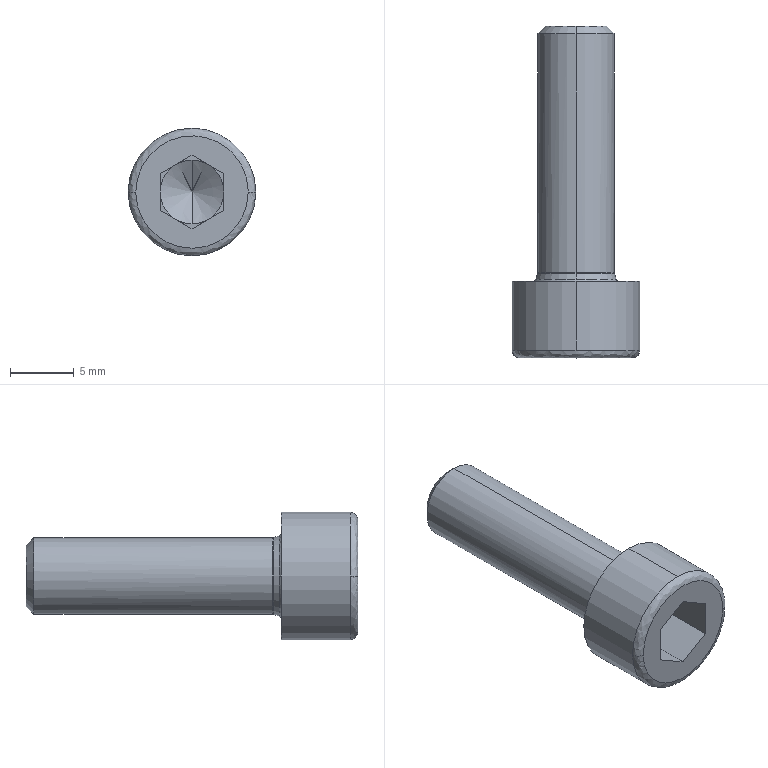Part | STEP file | 2_3 | 1 solid | 31 faces | box 10 x 26 x 10 mm | volume 942.975 mm3 | plane 15 | spline 6 | cone 6 | cylinder 4 | commonest cylinder face diameters 6 x2 10 x2